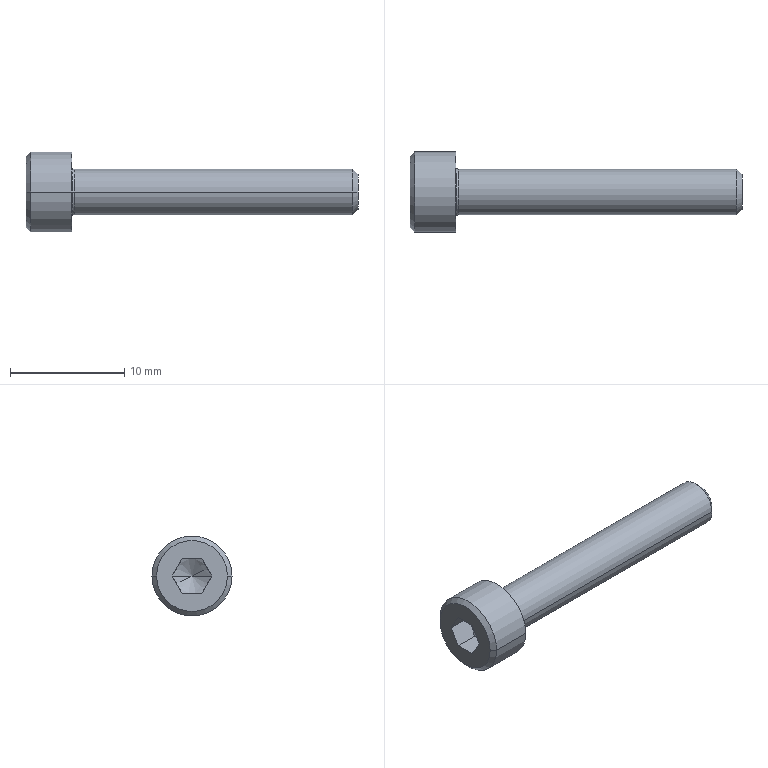Part | Creo | 1 solid | 23 faces | box 29 x 7 x 7 mm | volume 446.432 mm3 | plane 9 | cone 6 | cylinder 4 | torus 4 | commonest cylinder face diameters 4 x2 7 x2
STEP:
#1=CARTESIAN_POINT('',(0.,0.,0.));
#2=DIRECTION('',(0.,0.,1.));
#3=DIRECTION('',(1.,0.,0.));
#4=AXIS2_PLACEMENT_3D('',#1,#2,#3);
#5=CARTESIAN_POINT('',(-196.9,175.518,-24.));
#6=VERTEX_POINT('',#5);
#7=CARTESIAN_POINT('',(-196.9,176.384,-22.5));
#8=VERTEX_POINT('',#7);
#9=CARTESIAN_POINT('',(-196.9,175.518,-24.));
#10=CARTESIAN_POINT('',(-196.873,175.565,-23.918));
#11=CARTESIAN_POINT('',(-196.825,175.66,-23.754));
#12=CARTESIAN_POINT('',(-196.777,175.805,-23.503));
#13=CARTESIAN_POINT('',(-196.76,175.951,-23.249));
#14=CARTESIAN_POINT('',(-196.777,176.098,-22.996));
#15=CARTESIAN_POINT('',(-196.825,176.243,-22.745));
#16=CARTESIAN_POINT('',(-196.873,176.337,-22.581));
#17=CARTESIAN_POINT('',(-196.9,176.384,-22.5));
#18=B_SPLINE_CURVE_WITH_KNOTS('',3,(#9,#10,#11,#12,#13,#14,#15,#16,#17),.UNSPECIFIED.,.F.,.F.,(4,1,1,1,1,1,4),(0.,0.1667,0.3333,0.5,0.6667,0.8333,1.),.UNSPECIFIED.);
#19=EDGE_CURVE('',#6,#8,#18,.T.);
#20=ORIENTED_EDGE('',*,*,#19,.F.);
#21=CARTESIAN_POINT('',(-195.9,177.25,-24.));
#22=VERTEX_POINT('',#21);
#23=CARTESIAN_POINT('',(-195.9,177.25,-24.));
#24=DIRECTION('',(-0.5,-0.866,0.));
#25=VECTOR('',#24,2.);
#26=LINE('',#23,#25);
#27=EDGE_CURVE('',#22,#6,#26,.T.);
#28=ORIENTED_EDGE('',*,*,#27,.F.);
#29=CARTESIAN_POINT('',(-196.9,178.982,-24.));
#30=VERTEX_POINT('',#29);
#31=CARTESIAN_POINT('',(-195.9,177.25,-24.));
#32=DIRECTION('',(-0.5,0.866,0.));
#33=VECTOR('',#32,2.);
#34=LINE('',#31,#33);
#35=EDGE_CURVE('',#22,#30,#34,.T.);
#36=ORIENTED_EDGE('',*,*,#35,.T.);
#37=CARTESIAN_POINT('',(-196.9,178.116,-22.5));
#38=VERTEX_POINT('',#37);
#39=CARTESIAN_POINT('',(-196.9,178.116,-22.5));
#40=CARTESIAN_POINT('',(-196.873,178.163,-22.582));
#41=CARTESIAN_POINT('',(-196.825,178.258,-22.746));
#42=CARTESIAN_POINT('',(-196.777,178.403,-22.997));
#43=CARTESIAN_POINT('',(-196.76,178.549,-23.251));
#44=CARTESIAN_POINT('',(-196.777,178.696,-23.504));
#45=CARTESIAN_POINT('',(-196.825,178.841,-23.755));
#46=CARTESIAN_POINT('',(-196.873,178.935,-23.919));
#47=CARTESIAN_POINT('',(-196.9,178.982,-24.));
#48=B_SPLINE_CURVE_WITH_KNOTS('',3,(#39,#40,#41,#42,#43,#44,#45,#46,#47),.UNSPECIFIED.,.F.,.F.,(4,1,1,1,1,1,4),(0.,0.1667,0.3333,0.5,0.6667,0.8333,1.),.UNSPECIFIED.);
#49=EDGE_CURVE('',#38,#30,#48,.T.);
#50=ORIENTED_EDGE('',*,*,#49,.F.);
#51=CARTESIAN_POINT('',(-196.9,176.384,-22.5));
#52=CARTESIAN_POINT('',(-196.885,176.435,-22.5));
#53=CARTESIAN_POINT('',(-196.859,176.534,-22.5));
#54=CARTESIAN_POINT('',(-196.826,176.679,-22.5));
#55=CARTESIAN_POINT('',(-196.8,176.82,-22.5));
#56=CARTESIAN_POINT('',(-196.781,176.962,-22.5));
#57=CARTESIAN_POINT('',(-196.769,177.105,-22.5));
#58=CARTESIAN_POINT('',(-196.765,177.25,-22.5));
#59=CARTESIAN_POINT('',(-196.769,177.395,-22.5));
#60=CARTESIAN_POINT('',(-196.781,177.538,-22.5));
#61=CARTESIAN_POINT('',(-196.8,177.68,-22.5));
#62=CARTESIAN_POINT('',(-196.826,177.821,-22.5));
#63=CARTESIAN_POINT('',(-196.858,177.966,-22.5));
#64=CARTESIAN_POINT('',(-196.885,178.065,-22.5));
#65=CARTESIAN_POINT('',(-196.9,178.116,-22.5));
#66=B_SPLINE_CURVE_WITH_KNOTS('',3,(#51,#52,#53,#54,#55,#56,#57,#58,#59,#60,#61,#62,#63,#64,#65),.UNSPECIFIED.,.F.,.F.,(4,1,1,1,1,1,1,1,1,1,1,1,4),(0.,0.08333,0.1667,0.25,0.3333,0.4167,0.5,0.5833,0.6667,0.75,0.8333,0.9167,1.),.UNSPECIFIED.);
#67=EDGE_CURVE('',#8,#38,#66,.T.);
#68=ORIENTED_EDGE('',*,*,#67,.F.);
#69=EDGE_LOOP('',(#20,#28,#36,#50,#68));
#70=FACE_OUTER_BOUND('',#69,.F.);
#71=CARTESIAN_POINT('',(-196.41,177.25,-24.));
#72=DIRECTION('',(-1.,0.,0.));
#73=DIRECTION('',(0.,-1.,0.));
#74=AXIS2_PLACEMENT_3D('',#71,#72,#73);
#75=CONICAL_SURFACE('',#74,0.8833,60.);
#76=ADVANCED_FACE('',(#70),#75,.F.);
#77=CARTESIAN_POINT('',(-198.9,176.384,-22.5));
#78=VERTEX_POINT('',#77);
#79=CARTESIAN_POINT('',(-198.9,175.518,-24.));
#80=VERTEX_POINT('',#79);
#81=CARTESIAN_POINT('',(-198.9,176.384,-22.5));
#82=DIRECTION('',(0.,-0.5,-0.866));
#83=VECTOR('',#82,1.732);
#84=LINE('',#81,#83);
#85=EDGE_CURVE('',#78,#80,#84,.T.);
#86=ORIENTED_EDGE('',*,*,#85,.T.);
#87=CARTESIAN_POINT('',(-198.9,175.518,-24.));
#88=DIRECTION('',(1.,0.,0.));
#89=VECTOR('',#88,2.);
#90=LINE('',#87,#89);
#91=EDGE_CURVE('',#80,#6,#90,.T.);
#92=ORIENTED_EDGE('',*,*,#91,.T.);
#93=ORIENTED_EDGE('',*,*,#19,.T.);
#94=CARTESIAN_POINT('',(-198.9,176.384,-22.5));
#95=DIRECTION('',(1.,0.,0.));
#96=VECTOR('',#95,2.);
#97=LINE('',#94,#96);
#98=EDGE_CURVE('',#78,#8,#97,.T.);
#99=ORIENTED_EDGE('',*,*,#98,.F.);
#100=EDGE_LOOP('',(#86,#92,#93,#99));
#101=FACE_OUTER_BOUND('',#100,.F.);
#102=CARTESIAN_POINT('',(-196.9,176.384,-22.5));
#103=DIRECTION('',(0.,0.866,-0.5));
#104=DIRECTION('',(0.,-0.5,-0.866));
#105=AXIS2_PLACEMENT_3D('',#102,#103,#104);
#106=PLANE('',#105);
#107=ADVANCED_FACE('',(#101),#106,.T.);
#108=CARTESIAN_POINT('',(-198.9,174.15,-24.));
#109=VERTEX_POINT('',#108);
#110=CARTESIAN_POINT('',(-198.9,180.35,-24.));
#111=VERTEX_POINT('',#110);
#112=CARTESIAN_POINT('',(-198.9,177.25,-24.));
#113=DIRECTION('',(-1.,0.,0.));
#114=DIRECTION('',(0.,-1.,0.));
#115=AXIS2_PLACEMENT_3D('',#112,#113,#114);
#116=CIRCLE('',#115,3.1);
#117=EDGE_CURVE('',#109,#111,#116,.T.);
#118=ORIENTED_EDGE('',*,*,#117,.F.);
#119=CARTESIAN_POINT('',(-198.9,177.25,-24.));
#120=DIRECTION('',(-1.,0.,0.));
#121=DIRECTION('',(0.,1.,0.));
#122=AXIS2_PLACEMENT_3D('',#119,#120,#121);
#123=CIRCLE('',#122,3.1);
#124=EDGE_CURVE('',#111,#109,#123,.T.);
#125=ORIENTED_EDGE('',*,*,#124,.F.);
#126=EDGE_LOOP('',(#118,#125));
#127=FACE_OUTER_BOUND('',#126,.F.);
#128=CARTESIAN_POINT('',(-198.9,176.384,-25.5));
#129=VERTEX_POINT('',#128);
#130=CARTESIAN_POINT('',(-198.9,175.518,-24.));
#131=DIRECTION('',(0.,0.5,-0.866));
#132=VECTOR('',#131,1.732);
#133=LINE('',#130,#132);
#134=EDGE_CURVE('',#80,#129,#133,.T.);
#135=ORIENTED_EDGE('',*,*,#134,.F.);
#136=ORIENTED_EDGE('',*,*,#85,.F.);
#137=CARTESIAN_POINT('',(-198.9,178.116,-22.5));
#138=VERTEX_POINT('',#137);
#139=CARTESIAN_POINT('',(-198.9,176.384,-22.5));
#140=DIRECTION('',(0.,1.,0.));
#141=VECTOR('',#140,1.732);
#142=LINE('',#139,#141);
#143=EDGE_CURVE('',#78,#138,#142,.T.);
#144=ORIENTED_EDGE('',*,*,#143,.T.);
#145=CARTESIAN_POINT('',(-198.9,178.982,-24.));
#146=VERTEX_POINT('',#145);
#147=CARTESIAN_POINT('',(-198.9,178.982,-24.));
#148=DIRECTION('',(0.,-0.5,0.866));
#149=VECTOR('',#148,1.732);
#150=LINE('',#147,#149);
#151=EDGE_CURVE('',#146,#138,#150,.T.);
#152=ORIENTED_EDGE('',*,*,#151,.F.);
#153=CARTESIAN_POINT('',(-198.9,178.116,-25.5));
#154=VERTEX_POINT('',#153);
#155=CARTESIAN_POINT('',(-198.9,178.116,-25.5));
#156=DIRECTION('',(0.,0.5,0.866));
#157=VECTOR('',#156,1.732);
#158=LINE('',#155,#157);
#159=EDGE_CURVE('',#154,#146,#158,.T.);
#160=ORIENTED_EDGE('',*,*,#159,.F.);
#161=CARTESIAN_POINT('',(-198.9,178.116,-25.5));
#162=DIRECTION('',(0.,-1.,0.));
#163=VECTOR('',#162,1.732);
#164=LINE('',#161,#163);
#165=EDGE_CURVE('',#154,#129,#164,.T.);
#166=ORIENTED_EDGE('',*,*,#165,.T.);
#167=EDGE_LOOP('',(#135,#136,#144,#152,#160,#166));
#168=FACE_BOUND('',#167,.F.);
#169=CARTESIAN_POINT('',(-198.9,177.25,-24.));
#170=DIRECTION('',(-1.,0.,0.));
#171=DIRECTION('',(0.,-1.,0.));
#172=AXIS2_PLACEMENT_3D('',#169,#170,#171);
#173=PLANE('',#172);
#174=ADVANCED_FACE('',(#127,#168),#173,.T.);
#175=CARTESIAN_POINT('',(-198.5,173.75,-24.));
#176=VERTEX_POINT('',#175);
#177=CARTESIAN_POINT('',(-198.5,180.75,-24.));
#178=VERTEX_POINT('',#177);
#179=CARTESIAN_POINT('',(-198.5,177.25,-24.));
#180=DIRECTION('',(-1.,0.,0.));
#181=DIRECTION('',(0.,-1.,0.));
#182=AXIS2_PLACEMENT_3D('',#179,#180,#181);
#183=CIRCLE('',#182,3.5);
#184=EDGE_CURVE('',#176,#178,#183,.T.);
#185=ORIENTED_EDGE('',*,*,#184,.F.);
#186=CARTESIAN_POINT('',(-198.9,174.15,-24.));
#187=DIRECTION('',(0.7071,-0.7071,0.));
#188=VECTOR('',#187,0.5657);
#189=LINE('',#186,#188);
#190=EDGE_CURVE('',#109,#176,#189,.T.);
#191=ORIENTED_EDGE('',*,*,#190,.F.);
#192=ORIENTED_EDGE('',*,*,#117,.T.);
#193=CARTESIAN_POINT('',(-198.9,180.35,-24.));
#194=DIRECTION('',(0.7071,0.7071,0.));
#195=VECTOR('',#194,0.5657);
#196=LINE('',#193,#195);
#197=EDGE_CURVE('',#111,#178,#196,.T.);
#198=ORIENTED_EDGE('',*,*,#197,.T.);
#199=EDGE_LOOP('',(#185,#191,#192,#198));
#200=FACE_OUTER_BOUND('',#199,.F.);
#201=CARTESIAN_POINT('',(-198.7,177.25,-24.));
#202=DIRECTION('',(1.,0.,0.));
#203=DIRECTION('',(0.,1.,0.));
#204=AXIS2_PLACEMENT_3D('',#201,#202,#203);
#205=CONICAL_SURFACE('',#204,3.3,45.);
#206=ADVANCED_FACE('',(#200),#205,.T.);
#207=ORIENTED_EDGE('',*,*,#184,.T.);
#208=CARTESIAN_POINT('',(-194.9,180.75,-24.));
#209=VERTEX_POINT('',#208);
#210=CARTESIAN_POINT('',(-194.9,180.75,-24.));
#211=DIRECTION('',(-1.,0.,0.));
#212=VECTOR('',#211,3.6);
#213=LINE('',#210,#212);
#214=EDGE_CURVE('',#209,#178,#213,.T.);
#215=ORIENTED_EDGE('',*,*,#214,.F.);
#216=CARTESIAN_POINT('',(-194.9,173.75,-24.));
#217=VERTEX_POINT('',#216);
#218=CARTESIAN_POINT('',(-194.9,177.25,-24.));
#219=DIRECTION('',(1.,0.,0.));
#220=DIRECTION('',(0.,1.,0.));
#221=AXIS2_PLACEMENT_3D('',#218,#219,#220);
#222=CIRCLE('',#221,3.5);
#223=EDGE_CURVE('',#209,#217,#222,.T.);
#224=ORIENTED_EDGE('',*,*,#223,.T.);
#225=CARTESIAN_POINT('',(-194.9,173.75,-24.));
#226=DIRECTION('',(-1.,0.,0.));
#227=VECTOR('',#226,3.6);
#228=LINE('',#225,#227);
#229=EDGE_CURVE('',#217,#176,#228,.T.);
#230=ORIENTED_EDGE('',*,*,#229,.T.);
#231=EDGE_LOOP('',(#207,#215,#224,#230));
#232=FACE_OUTER_BOUND('',#231,.F.);
#233=CARTESIAN_POINT('',(-194.9,177.25,-24.));
#234=DIRECTION('',(-1.,0.,0.));
#235=DIRECTION('',(0.,-1.,0.));
#236=AXIS2_PLACEMENT_3D('',#233,#234,#235);
#237=CYLINDRICAL_SURFACE('',#236,3.5);
#238=ADVANCED_FACE('',(#232),#237,.T.);
#239=CARTESIAN_POINT('',(-198.5,177.25,-24.));
#240=DIRECTION('',(-1.,0.,0.));
#241=DIRECTION('',(0.,1.,0.));
#242=AXIS2_PLACEMENT_3D('',#239,#240,#241);
#243=CIRCLE('',#242,3.5);
#244=EDGE_CURVE('',#178,#176,#243,.T.);
#245=ORIENTED_EDGE('',*,*,#244,.T.);
#246=ORIENTED_EDGE('',*,*,#229,.F.);
#247=CARTESIAN_POINT('',(-194.9,177.25,-24.));
#248=DIRECTION('',(1.,0.,0.));
#249=DIRECTION('',(0.,-1.,0.));
#250=AXIS2_PLACEMENT_3D('',#247,#248,#249);
#251=CIRCLE('',#250,3.5);
#252=EDGE_CURVE('',#217,#209,#251,.T.);
#253=ORIENTED_EDGE('',*,*,#252,.T.);
#254=ORIENTED_EDGE('',*,*,#214,.T.);
#255=EDGE_LOOP('',(#245,#246,#253,#254));
#256=FACE_OUTER_BOUND('',#255,.F.);
#257=CARTESIAN_POINT('',(-194.9,177.25,-24.));
#258=DIRECTION('',(-1.,0.,0.));
#259=DIRECTION('',(0.,-1.,0.));
#260=AXIS2_PLACEMENT_3D('',#257,#258,#259);
#261=CYLINDRICAL_SURFACE('',#260,3.5);
#262=ADVANCED_FACE('',(#256),#261,.T.);
#263=ORIENTED_EDGE('',*,*,#244,.F.);
#264=ORIENTED_EDGE('',*,*,#197,.F.);
#265=ORIENTED_EDGE('',*,*,#124,.T.);
#266=ORIENTED_EDGE('',*,*,#190,.T.);
#267=EDGE_LOOP('',(#263,#264,#265,#266));
#268=FACE_OUTER_BOUND('',#267,.F.);
#269=CARTESIAN_POINT('',(-198.7,177.25,-24.));
#270=DIRECTION('',(1.,0.,0.));
#271=DIRECTION('',(0.,1.,0.));
#272=AXIS2_PLACEMENT_3D('',#269,#270,#271);
#273=CONICAL_SURFACE('',#272,3.3,45.);
#274=ADVANCED_FACE('',(#268),#273,.T.);
#275=ORIENTED_EDGE('',*,*,#252,.F.);
#276=ORIENTED_EDGE('',*,*,#223,.F.);
#277=EDGE_LOOP('',(#275,#276));
#278=FACE_OUTER_BOUND('',#277,.F.);
#279=CARTESIAN_POINT('',(-194.9,175.05,-24.));
#280=VERTEX_POINT('',#279);
#281=CARTESIAN_POINT('',(-194.9,179.45,-24.));
#282=VERTEX_POINT('',#281);
#283=CARTESIAN_POINT('',(-194.9,177.25,-24.));
#284=DIRECTION('',(-1.,0.,0.));
#285=DIRECTION('',(0.,-1.,0.));
#286=AXIS2_PLACEMENT_3D('',#283,#284,#285);
#287=CIRCLE('',#286,2.2);
#288=EDGE_CURVE('',#280,#282,#287,.T.);
#289=ORIENTED_EDGE('',*,*,#288,.F.);
#290=CARTESIAN_POINT('',(-194.9,177.25,-24.));
#291=DIRECTION('',(-1.,0.,0.));
#292=DIRECTION('',(0.,1.,0.));
#293=AXIS2_PLACEMENT_3D('',#290,#291,#292);
#294=CIRCLE('',#293,2.2);
#295=EDGE_CURVE('',#282,#280,#294,.T.);
#296=ORIENTED_EDGE('',*,*,#295,.F.);
#297=EDGE_LOOP('',(#289,#296));
#298=FACE_BOUND('',#297,.F.);
#299=CARTESIAN_POINT('',(-194.9,177.25,-24.));
#300=DIRECTION('',(-1.,0.,0.));
#301=DIRECTION('',(0.,-1.,0.));
#302=AXIS2_PLACEMENT_3D('',#299,#300,#301);
#303=PLANE('',#302);
#304=ADVANCED_FACE('',(#278,#298),#303,.F.);
#305=ORIENTED_EDGE('',*,*,#288,.T.);
#306=CARTESIAN_POINT('',(-194.841,179.309,-24.));
#307=VERTEX_POINT('',#306);
#308=CARTESIAN_POINT('',(-194.7,179.45,-24.));
#309=DIRECTION('',(0.,0.,1.));
#310=DIRECTION('',(-1.,0.,0.));
#311=AXIS2_PLACEMENT_3D('',#308,#309,#310);
#312=CIRCLE('',#311,0.2);
#313=EDGE_CURVE('',#282,#307,#312,.T.);
#314=ORIENTED_EDGE('',*,*,#313,.T.);
#315=CARTESIAN_POINT('',(-194.841,175.191,-24.));
#316=VERTEX_POINT('',#315);
#317=CARTESIAN_POINT('',(-194.841,177.25,-24.));
#318=DIRECTION('',(-1.,0.,0.));
#319=DIRECTION('',(0.,-1.,0.));
#320=AXIS2_PLACEMENT_3D('',#317,#318,#319);
#321=CIRCLE('',#320,2.059);
#322=EDGE_CURVE('',#316,#307,#321,.T.);
#323=ORIENTED_EDGE('',*,*,#322,.F.);
#324=CARTESIAN_POINT('',(-194.7,175.05,-24.));
#325=DIRECTION('',(0.,0.,-1.));
#326=DIRECTION('',(-1.,0.,0.));
#327=AXIS2_PLACEMENT_3D('',#324,#325,#326);
#328=CIRCLE('',#327,0.2);
#329=EDGE_CURVE('',#280,#316,#328,.T.);
#330=ORIENTED_EDGE('',*,*,#329,.F.);
#331=EDGE_LOOP('',(#305,#314,#323,#330));
#332=FACE_OUTER_BOUND('',#331,.F.);
#333=CARTESIAN_POINT('',(-194.7,177.25,-24.));
#334=DIRECTION('',(-1.,0.,0.));
#335=DIRECTION('',(0.,-1.,0.));
#336=AXIS2_PLACEMENT_3D('',#333,#334,#335);
#337=TOROIDAL_SURFACE('',#336,2.2,0.2);
#338=ADVANCED_FACE('',(#332),#337,.F.);
#339=ORIENTED_EDGE('',*,*,#295,.T.);
#340=ORIENTED_EDGE('',*,*,#329,.T.);
#341=CARTESIAN_POINT('',(-194.841,177.25,-24.));
#342=DIRECTION('',(-1.,0.,0.));
#343=DIRECTION('',(0.,1.,0.));
#344=AXIS2_PLACEMENT_3D('',#341,#342,#343);
#345=CIRCLE('',#344,2.059);
#346=EDGE_CURVE('',#307,#316,#345,.T.);
#347=ORIENTED_EDGE('',*,*,#346,.F.);
#348=ORIENTED_EDGE('',*,*,#313,.F.);
#349=EDGE_LOOP('',(#339,#340,#347,#348));
#350=FACE_OUTER_BOUND('',#349,.F.);
#351=CARTESIAN_POINT('',(-194.7,177.25,-24.));
#352=DIRECTION('',(-1.,0.,0.));
#353=DIRECTION('',(0.,-1.,0.));
#354=AXIS2_PLACEMENT_3D('',#351,#352,#353);
#355=TOROIDAL_SURFACE('',#354,2.2,0.2);
#356=ADVANCED_FACE('',(#350),#355,.F.);
#357=CARTESIAN_POINT('',(-194.7,179.25,-24.));
#358=VERTEX_POINT('',#357);
#359=CARTESIAN_POINT('',(-194.7,175.25,-24.));
#360=VERTEX_POINT('',#359);
#361=CARTESIAN_POINT('',(-194.7,177.25,-24.));
#362=DIRECTION('',(-1.,0.,0.));
#363=DIRECTION('',(0.,1.,0.));
#364=AXIS2_PLACEMENT_3D('',#361,#362,#363);
#365=CIRCLE('',#364,2.);
#366=EDGE_CURVE('',#358,#360,#365,.T.);
#367=ORIENTED_EDGE('',*,*,#366,.F.);
#368=CARTESIAN_POINT('',(-194.7,179.45,-24.));
#369=DIRECTION('',(0.,0.,1.));
#370=DIRECTION('',(-0.7071,-0.7071,0.));
#371=AXIS2_PLACEMENT_3D('',#368,#369,#370);
#372=CIRCLE('',#371,0.2);
#373=EDGE_CURVE('',#307,#358,#372,.T.);
#374=ORIENTED_EDGE('',*,*,#373,.F.);
#375=ORIENTED_EDGE('',*,*,#346,.T.);
#376=CARTESIAN_POINT('',(-194.7,175.05,-24.));
#377=DIRECTION('',(0.,0.,-1.));
#378=DIRECTION('',(-0.7071,0.7071,0.));
#379=AXIS2_PLACEMENT_3D('',#376,#377,#378);
#380=CIRCLE('',#379,0.2);
#381=EDGE_CURVE('',#316,#360,#380,.T.);
#382=ORIENTED_EDGE('',*,*,#381,.T.);
#383=EDGE_LOOP('',(#367,#374,#375,#382));
#384=FACE_OUTER_BOUND('',#383,.F.);
#385=CARTESIAN_POINT('',(-194.7,177.25,-24.));
#386=DIRECTION('',(-1.,0.,0.));
#387=DIRECTION('',(0.,-1.,0.));
#388=AXIS2_PLACEMENT_3D('',#385,#386,#387);
#389=TOROIDAL_SURFACE('',#388,2.2,0.2);
#390=ADVANCED_FACE('',(#384),#389,.F.);
#391=CARTESIAN_POINT('',(-170.4,175.25,-24.));
#392=VERTEX_POINT('',#391);
#393=CARTESIAN_POINT('',(-170.4,179.25,-24.));
#394=VERTEX_POINT('',#393);
#395=CARTESIAN_POINT('',(-170.4,177.25,-24.));
#396=DIRECTION('',(1.,0.,0.));
#397=DIRECTION('',(0.,-1.,0.));
#398=AXIS2_PLACEMENT_3D('',#395,#396,#397);
#399=CIRCLE('',#398,2.);
#400=EDGE_CURVE('',#392,#394,#399,.T.);
#401=ORIENTED_EDGE('',*,*,#400,.T.);
#402=CARTESIAN_POINT('',(-170.4,179.25,-24.));
#403=DIRECTION('',(-1.,0.,0.));
#404=VECTOR('',#403,24.3);
#405=LINE('',#402,#404);
#406=EDGE_CURVE('',#394,#358,#405,.T.);
#407=ORIENTED_EDGE('',*,*,#406,.T.);
#408=ORIENTED_EDGE('',*,*,#366,.T.);
#409=CARTESIAN_POINT('',(-170.4,175.25,-24.));
#410=DIRECTION('',(-1.,0.,0.));
#411=VECTOR('',#410,24.3);
#412=LINE('',#409,#411);
#413=EDGE_CURVE('',#392,#360,#412,.T.);
#414=ORIENTED_EDGE('',*,*,#413,.F.);
#415=EDGE_LOOP('',(#401,#407,#408,#414));
#416=FACE_OUTER_BOUND('',#415,.F.);
#417=CARTESIAN_POINT('',(-169.9,177.25,-24.));
#418=DIRECTION('',(-1.,0.,0.));
#419=DIRECTION('',(0.,-1.,0.));
#420=AXIS2_PLACEMENT_3D('',#417,#418,#419);
#421=CYLINDRICAL_SURFACE('',#420,2.);
#422=ADVANCED_FACE('',(#416),#421,.T.);
#423=CARTESIAN_POINT('',(-169.9,175.75,-24.));
#424=VERTEX_POINT('',#423);
#425=CARTESIAN_POINT('',(-169.9,178.75,-24.));
#426=VERTEX_POINT('',#425);
#427=CARTESIAN_POINT('',(-169.9,177.25,-24.));
#428=DIRECTION('',(1.,0.,0.));
#429=DIRECTION('',(0.,-1.,0.));
#430=AXIS2_PLACEMENT_3D('',#427,#428,#429);
#431=CIRCLE('',#430,1.5);
#432=EDGE_CURVE('',#424,#426,#431,.T.);
#433=ORIENTED_EDGE('',*,*,#432,.T.);
#434=CARTESIAN_POINT('',(-169.9,178.75,-24.));
#435=DIRECTION('',(-0.7071,0.7071,0.));
#436=VECTOR('',#435,0.7071);
#437=LINE('',#434,#436);
#438=EDGE_CURVE('',#426,#394,#437,.T.);
#439=ORIENTED_EDGE('',*,*,#438,.T.);
#440=ORIENTED_EDGE('',*,*,#400,.F.);
#441=CARTESIAN_POINT('',(-169.9,175.75,-24.));
#442=DIRECTION('',(-0.7071,-0.7071,0.));
#443=VECTOR('',#442,0.7071);
#444=LINE('',#441,#443);
#445=EDGE_CURVE('',#424,#392,#444,.T.);
#446=ORIENTED_EDGE('',*,*,#445,.F.);
#447=EDGE_LOOP('',(#433,#439,#440,#446));
#448=FACE_OUTER_BOUND('',#447,.F.);
#449=CARTESIAN_POINT('',(-170.15,177.25,-24.));
#450=DIRECTION('',(-1.,0.,0.));
#451=DIRECTION('',(0.,-1.,0.));
#452=AXIS2_PLACEMENT_3D('',#449,#450,#451);
#453=CONICAL_SURFACE('',#452,1.75,45.);
#454=ADVANCED_FACE('',(#448),#453,.T.);
#455=ORIENTED_EDGE('',*,*,#432,.F.);
#456=CARTESIAN_POINT('',(-169.9,177.25,-24.));
#457=DIRECTION('',(1.,0.,0.));
#458=DIRECTION('',(0.,1.,0.));
#459=AXIS2_PLACEMENT_3D('',#456,#457,#458);
#460=CIRCLE('',#459,1.5);
#461=EDGE_CURVE('',#426,#424,#460,.T.);
#462=ORIENTED_EDGE('',*,*,#461,.F.);
#463=EDGE_LOOP('',(#455,#462));
#464=FACE_OUTER_BOUND('',#463,.F.);
#465=CARTESIAN_POINT('',(-169.9,177.25,-24.));
#466=DIRECTION('',(-1.,0.,0.));
#467=DIRECTION('',(0.,-1.,0.));
#468=AXIS2_PLACEMENT_3D('',#465,#466,#467);
#469=PLANE('',#468);
#470=ADVANCED_FACE('',(#464),#469,.F.);
#471=ORIENTED_EDGE('',*,*,#461,.T.);
#472=ORIENTED_EDGE('',*,*,#445,.T.);
#473=CARTESIAN_POINT('',(-170.4,177.25,-24.));
#474=DIRECTION('',(1.,0.,0.));
#475=DIRECTION('',(0.,1.,0.));
#476=AXIS2_PLACEMENT_3D('',#473,#474,#475);
#477=CIRCLE('',#476,2.);
#478=EDGE_CURVE('',#394,#392,#477,.T.);
#479=ORIENTED_EDGE('',*,*,#478,.F.);
#480=ORIENTED_EDGE('',*,*,#438,.F.);
#481=EDGE_LOOP('',(#471,#472,#479,#480));
#482=FACE_OUTER_BOUND('',#481,.F.);
#483=CARTESIAN_POINT('',(-170.15,177.25,-24.));
#484=DIRECTION('',(-1.,0.,0.));
#485=DIRECTION('',(0.,-1.,0.));
#486=AXIS2_PLACEMENT_3D('',#483,#484,#485);
#487=CONICAL_SURFACE('',#486,1.75,45.);
#488=ADVANCED_FACE('',(#482),#487,.T.);
#489=ORIENTED_EDGE('',*,*,#478,.T.);
#490=ORIENTED_EDGE('',*,*,#413,.T.);
#491=CARTESIAN_POINT('',(-194.7,177.25,-24.));
#492=DIRECTION('',(-1.,0.,0.));
#493=DIRECTION('',(0.,-1.,0.));
#494=AXIS2_PLACEMENT_3D('',#491,#492,#493);
#495=CIRCLE('',#494,2.);
#496=EDGE_CURVE('',#360,#358,#495,.T.);
#497=ORIENTED_EDGE('',*,*,#496,.T.);
#498=ORIENTED_EDGE('',*,*,#406,.F.);
#499=EDGE_LOOP('',(#489,#490,#497,#498));
#500=FACE_OUTER_BOUND('',#499,.F.);
#501=CARTESIAN_POINT('',(-169.9,177.25,-24.));
#502=DIRECTION('',(-1.,0.,0.));
#503=DIRECTION('',(0.,-1.,0.));
#504=AXIS2_PLACEMENT_3D('',#501,#502,#503);
#505=CYLINDRICAL_SURFACE('',#504,2.);
#506=ADVANCED_FACE('',(#500),#505,.T.);
#507=ORIENTED_EDGE('',*,*,#496,.F.);
#508=ORIENTED_EDGE('',*,*,#381,.F.);
#509=ORIENTED_EDGE('',*,*,#322,.T.);
#510=ORIENTED_EDGE('',*,*,#373,.T.);
#511=EDGE_LOOP('',(#507,#508,#509,#510));
#512=FACE_OUTER_BOUND('',#511,.F.);
#513=CARTESIAN_POINT('',(-194.7,177.25,-24.));
#514=DIRECTION('',(-1.,0.,0.));
#515=DIRECTION('',(0.,-1.,0.));
#516=AXIS2_PLACEMENT_3D('',#513,#514,#515);
#517=TOROIDAL_SURFACE('',#516,2.2,0.2);
#518=ADVANCED_FACE('',(#512),#517,.F.);
#519=ORIENTED_EDGE('',*,*,#134,.T.);
#520=CARTESIAN_POINT('',(-196.9,176.384,-25.5));
#521=VERTEX_POINT('',#520);
#522=CARTESIAN_POINT('',(-198.9,176.384,-25.5));
#523=DIRECTION('',(1.,0.,0.));
#524=VECTOR('',#523,2.);
#525=LINE('',#522,#524);
#526=EDGE_CURVE('',#129,#521,#525,.T.);
#527=ORIENTED_EDGE('',*,*,#526,.T.);
#528=CARTESIAN_POINT('',(-196.9,176.384,-25.5));
#529=CARTESIAN_POINT('',(-196.873,176.337,-25.418));
#530=CARTESIAN_POINT('',(-196.825,176.242,-25.254));
#531=CARTESIAN_POINT('',(-196.777,176.097,-25.003));
#532=CARTESIAN_POINT('',(-196.76,175.951,-24.749));
#533=CARTESIAN_POINT('',(-196.777,175.804,-24.496));
#534=CARTESIAN_POINT('',(-196.825,175.659,-24.245));
#535=CARTESIAN_POINT('',(-196.873,175.565,-24.081));
#536=CARTESIAN_POINT('',(-196.9,175.518,-24.));
#537=B_SPLINE_CURVE_WITH_KNOTS('',3,(#528,#529,#530,#531,#532,#533,#534,#535,#536),.UNSPECIFIED.,.F.,.F.,(4,1,1,1,1,1,4),(0.,0.1667,0.3333,0.5,0.6667,0.8333,1.),.UNSPECIFIED.);
#538=EDGE_CURVE('',#521,#6,#537,.T.);
#539=ORIENTED_EDGE('',*,*,#538,.T.);
#540=ORIENTED_EDGE('',*,*,#91,.F.);
#541=EDGE_LOOP('',(#519,#527,#539,#540));
#542=FACE_OUTER_BOUND('',#541,.F.);
#543=CARTESIAN_POINT('',(-196.9,175.518,-24.));
#544=DIRECTION('',(0.,0.866,0.5));
#545=DIRECTION('',(0.,0.5,-0.866));
#546=AXIS2_PLACEMENT_3D('',#543,#544,#545);
#547=PLANE('',#546);
#548=ADVANCED_FACE('',(#542),#547,.T.);
#549=ORIENTED_EDGE('',*,*,#165,.F.);
#550=CARTESIAN_POINT('',(-196.9,178.116,-25.5));
#551=VERTEX_POINT('',#550);
#552=CARTESIAN_POINT('',(-198.9,178.116,-25.5));
#553=DIRECTION('',(1.,0.,0.));
#554=VECTOR('',#553,2.);
#555=LINE('',#552,#554);
#556=EDGE_CURVE('',#154,#551,#555,.T.);
#557=ORIENTED_EDGE('',*,*,#556,.T.);
#558=CARTESIAN_POINT('',(-196.9,178.116,-25.5));
#559=CARTESIAN_POINT('',(-196.885,178.065,-25.5));
#560=CARTESIAN_POINT('',(-196.858,177.966,-25.5));
#561=CARTESIAN_POINT('',(-196.826,177.821,-25.5));
#562=CARTESIAN_POINT('',(-196.8,177.68,-25.5));
#563=CARTESIAN_POINT('',(-196.781,177.538,-25.5));
#564=CARTESIAN_POINT('',(-196.769,177.395,-25.5));
#565=CARTESIAN_POINT('',(-196.765,177.25,-25.5));
#566=CARTESIAN_POINT('',(-196.769,177.105,-25.5));
#567=CARTESIAN_POINT('',(-196.781,176.962,-25.5));
#568=CARTESIAN_POINT('',(-196.8,176.82,-25.5));
#569=CARTESIAN_POINT('',(-196.826,176.679,-25.5));
#570=CARTESIAN_POINT('',(-196.859,176.534,-25.5));
#571=CARTESIAN_POINT('',(-196.885,176.435,-25.5));
#572=CARTESIAN_POINT('',(-196.9,176.384,-25.5));
#573=B_SPLINE_CURVE_WITH_KNOTS('',3,(#558,#559,#560,#561,#562,#563,#564,#565,#566,#567,#568,#569,#570,#571,#572),.UNSPECIFIED.,.F.,.F.,(4,1,1,1,1,1,1,1,1,1,1,1,4),(0.,0.08333,0.1667,0.25,0.3333,0.4167,0.5,0.5833,0.6667,0.75,0.8333,0.9167,1.),.UNSPECIFIED.);
#574=EDGE_CURVE('',#551,#521,#573,.T.);
#575=ORIENTED_EDGE('',*,*,#574,.T.);
#576=ORIENTED_EDGE('',*,*,#526,.F.);
#577=EDGE_LOOP('',(#549,#557,#575,#576));
#578=FACE_OUTER_BOUND('',#577,.F.);
#579=CARTESIAN_POINT('',(-196.9,176.384,-25.5));
#580=DIRECTION('',(0.,0.,1.));
#581=DIRECTION('',(-1.,0.,0.));
#582=AXIS2_PLACEMENT_3D('',#579,#580,#581);
#583=PLANE('',#582);
#584=ADVANCED_FACE('',(#578),#583,.T.);
#585=ORIENTED_EDGE('',*,*,#159,.T.);
#586=CARTESIAN_POINT('',(-198.9,178.982,-24.));
#587=DIRECTION('',(1.,0.,0.));
#588=VECTOR('',#587,2.);
#589=LINE('',#586,#588);
#590=EDGE_CURVE('',#146,#30,#589,.T.);
#591=ORIENTED_EDGE('',*,*,#590,.T.);
#592=CARTESIAN_POINT('',(-196.9,178.982,-24.));
#593=CARTESIAN_POINT('',(-196.873,178.935,-24.081));
#594=CARTESIAN_POINT('',(-196.825,178.841,-24.245));
#595=CARTESIAN_POINT('',(-196.777,178.696,-24.496));
#596=CARTESIAN_POINT('',(-196.76,178.549,-24.749));
#597=CARTESIAN_POINT('',(-196.777,178.403,-25.003));
#598=CARTESIAN_POINT('',(-196.825,178.258,-25.254));
#599=CARTESIAN_POINT('',(-196.873,178.163,-25.418));
#600=CARTESIAN_POINT('',(-196.9,178.116,-25.5));
#601=B_SPLINE_CURVE_WITH_KNOTS('',3,(#592,#593,#594,#595,#596,#597,#598,#599,#600),.UNSPECIFIED.,.F.,.F.,(4,1,1,1,1,1,4),(0.,0.1667,0.3333,0.5,0.6667,0.8333,1.),.UNSPECIFIED.);
#602=EDGE_CURVE('',#30,#551,#601,.T.);
#603=ORIENTED_EDGE('',*,*,#602,.T.);
#604=ORIENTED_EDGE('',*,*,#556,.F.);
#605=EDGE_LOOP('',(#585,#591,#603,#604));
#606=FACE_OUTER_BOUND('',#605,.F.);
#607=CARTESIAN_POINT('',(-196.9,178.116,-25.5));
#608=DIRECTION('',(0.,-0.866,0.5));
#609=DIRECTION('',(0.,0.5,0.866));
#610=AXIS2_PLACEMENT_3D('',#607,#608,#609);
#611=PLANE('',#610);
#612=ADVANCED_FACE('',(#606),#611,.T.);
#613=ORIENTED_EDGE('',*,*,#151,.T.);
#614=CARTESIAN_POINT('',(-198.9,178.116,-22.5));
#615=DIRECTION('',(1.,0.,0.));
#616=VECTOR('',#615,2.);
#617=LINE('',#614,#616);
#618=EDGE_CURVE('',#138,#38,#617,.T.);
#619=ORIENTED_EDGE('',*,*,#618,.T.);
#620=ORIENTED_EDGE('',*,*,#49,.T.);
#621=ORIENTED_EDGE('',*,*,#590,.F.);
#622=EDGE_LOOP('',(#613,#619,#620,#621));
#623=FACE_OUTER_BOUND('',#622,.F.);
#624=CARTESIAN_POINT('',(-196.9,178.982,-24.));
#625=DIRECTION('',(0.,-0.866,-0.5));
#626=DIRECTION('',(0.,-0.5,0.866));
#627=AXIS2_PLACEMENT_3D('',#624,#625,#626);
#628=PLANE('',#627);
#629=ADVANCED_FACE('',(#623),#628,.T.);
#630=ORIENTED_EDGE('',*,*,#143,.F.);
#631=ORIENTED_EDGE('',*,*,#98,.T.);
#632=ORIENTED_EDGE('',*,*,#67,.T.);
#633=ORIENTED_EDGE('',*,*,#618,.F.);
#634=EDGE_LOOP('',(#630,#631,#632,#633));
#635=FACE_OUTER_BOUND('',#634,.F.);
#636=CARTESIAN_POINT('',(-196.9,178.116,-22.5));
#637=DIRECTION('',(0.,0.,-1.));
#638=DIRECTION('',(1.,0.,0.));
#639=AXIS2_PLACEMENT_3D('',#636,#637,#638);
#640=PLANE('',#639);
#641=ADVANCED_FACE('',(#635),#640,.T.);
#642=ORIENTED_EDGE('',*,*,#602,.F.);
#643=ORIENTED_EDGE('',*,*,#35,.F.);
#644=ORIENTED_EDGE('',*,*,#27,.T.);
#645=ORIENTED_EDGE('',*,*,#538,.F.);
#646=ORIENTED_EDGE('',*,*,#574,.F.);
#647=EDGE_LOOP('',(#642,#643,#644,#645,#646));
#648=FACE_OUTER_BOUND('',#647,.F.);
#649=CARTESIAN_POINT('',(-196.41,177.25,-24.));
#650=DIRECTION('',(-1.,0.,0.));
#651=DIRECTION('',(0.,-1.,0.));
#652=AXIS2_PLACEMENT_3D('',#649,#650,#651);
#653=CONICAL_SURFACE('',#652,0.8833,60.);
#654=ADVANCED_FACE('',(#648),#653,.F.);
#655=CLOSED_SHELL('',(#76,#107,#174,#206,#238,#262,#274,#304,#338,#356,#390,#422,#454,#470,#488,#506,#518,#548,#584,#612,#629,#641,#654));
#656=MANIFOLD_SOLID_BREP('',#655);
#657=(LENGTH_UNIT()NAMED_UNIT(*)SI_UNIT(.MILLI.,.METRE.));
#658=UNCERTAINTY_MEASURE_WITH_UNIT(LENGTH_MEASURE(0.003064),#657,'','');
#659=(NAMED_UNIT(*)PLANE_ANGLE_UNIT()SI_UNIT($,.RADIAN.));
#660=PLANE_ANGLE_MEASURE_WITH_UNIT(PLANE_ANGLE_MEASURE(0.01745),#659);
#661=(CONVERSION_BASED_UNIT('DEGREE',#660)NAMED_UNIT(*)PLANE_ANGLE_UNIT());
#662=(NAMED_UNIT(*)SI_UNIT($,.STERADIAN.)SOLID_ANGLE_UNIT());
#663=(GEOMETRIC_REPRESENTATION_CONTEXT(3)GLOBAL_UNCERTAINTY_ASSIGNED_CONTEXT((#658))GLOBAL_UNIT_ASSIGNED_CONTEXT((#657,#661,#662))REPRESENTATION_CONTEXT('',''));
#664=ADVANCED_BREP_SHAPE_REPRESENTATION('',(#4,#656),#663);